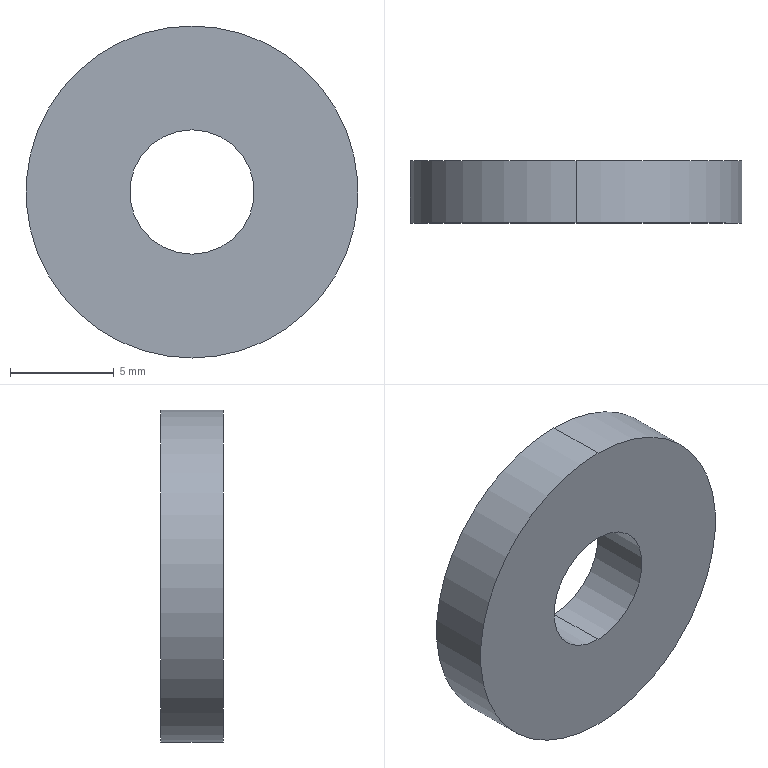Part | STEP file | PN_0004_default | 1 solid | 6 faces | box 16 x 3 x 16 mm | volume 518.363 mm3 | cylinder 4 | plane 2 | commonest cylinder face diameters 6 x2 16 x2
STEP:
#1=CARTESIAN_POINT('',(0.,0.,0.));
#2=DIRECTION('',(0.,0.,1.));
#3=DIRECTION('',(1.,0.,0.));
#4=AXIS2_PLACEMENT_3D('',#1,#2,#3);
#5=CARTESIAN_POINT('',(0.,3.,-3.));
#6=VERTEX_POINT('',#5);
#7=CARTESIAN_POINT('',(0.,0.,-3.));
#8=VERTEX_POINT('',#7);
#9=CARTESIAN_POINT('',(0.,3.,-3.));
#10=DIRECTION('',(0.,-1.,0.));
#11=VECTOR('',#10,1.);
#12=LINE('',#9,#11);
#13=CARTESIAN_POINT('',(0.,3.,0.));
#14=DIRECTION('',(0.,-1.,0.));
#15=DIRECTION('',(0.,0.,-1.));
#16=AXIS2_PLACEMENT_3D('',#13,#14,#15);
#17=CYLINDRICAL_SURFACE('',#16,3.);
#18=CARTESIAN_POINT('',(6.283,0.));
#19=DIRECTION('',(0.,1.));
#20=VECTOR('',#19,1.);
#21=LINE('',#18,#20);
#22=(GEOMETRIC_REPRESENTATION_CONTEXT(2)PARAMETRIC_REPRESENTATION_CONTEXT()REPRESENTATION_CONTEXT('',''));
#23=DEFINITIONAL_REPRESENTATION('',(#21),#22);
#24=PCURVE('',#17,#23);
#25=CARTESIAN_POINT('',(0.,3.,0.));
#26=DIRECTION('',(0.,-1.,0.));
#27=DIRECTION('',(0.,0.,-1.));
#28=AXIS2_PLACEMENT_3D('',#25,#26,#27);
#29=CYLINDRICAL_SURFACE('',#28,3.);
#30=CARTESIAN_POINT('',(0.,0.));
#31=DIRECTION('',(0.,1.));
#32=VECTOR('',#31,1.);
#33=LINE('',#30,#32);
#34=(GEOMETRIC_REPRESENTATION_CONTEXT(2)PARAMETRIC_REPRESENTATION_CONTEXT()REPRESENTATION_CONTEXT('',''));
#35=DEFINITIONAL_REPRESENTATION('',(#33),#34);
#36=PCURVE('',#29,#35);
#37=SURFACE_CURVE('',#12,(#24,#36),.PCURVE_S1.);
#38=EDGE_CURVE('',#6,#8,#37,.T.);
#39=ORIENTED_EDGE('',*,*,#38,.T.);
#40=CARTESIAN_POINT('',(0.,0.,3.));
#41=VERTEX_POINT('',#40);
#42=CARTESIAN_POINT('',(0.,0.,0.));
#43=DIRECTION('',(0.,1.,0.));
#44=DIRECTION('',(0.,0.,1.));
#45=AXIS2_PLACEMENT_3D('',#42,#43,#44);
#46=CIRCLE('',#45,3.);
#47=CARTESIAN_POINT('',(9.425,3.));
#48=DIRECTION('',(-1.,0.));
#49=VECTOR('',#48,1.);
#50=LINE('',#47,#49);
#51=(GEOMETRIC_REPRESENTATION_CONTEXT(2)PARAMETRIC_REPRESENTATION_CONTEXT()REPRESENTATION_CONTEXT('',''));
#52=DEFINITIONAL_REPRESENTATION('',(#50),#51);
#53=PCURVE('',#17,#52);
#54=CARTESIAN_POINT('',(0.,0.,0.));
#55=DIRECTION('',(0.,1.,0.));
#56=DIRECTION('',(0.,0.,1.));
#57=AXIS2_PLACEMENT_3D('',#54,#55,#56);
#58=PLANE('',#57);
#59=CARTESIAN_POINT('',(0.,0.));
#60=DIRECTION('',(1.,0.));
#61=AXIS2_PLACEMENT_2D('',#59,#60);
#62=CIRCLE('',#61,3.);
#63=(GEOMETRIC_REPRESENTATION_CONTEXT(2)PARAMETRIC_REPRESENTATION_CONTEXT()REPRESENTATION_CONTEXT('',''));
#64=DEFINITIONAL_REPRESENTATION('',(#62),#63);
#65=PCURVE('',#58,#64);
#66=SURFACE_CURVE('',#46,(#53,#65),.PCURVE_S1.);
#67=EDGE_CURVE('',#8,#41,#66,.T.);
#68=ORIENTED_EDGE('',*,*,#67,.T.);
#69=CARTESIAN_POINT('',(0.,3.,3.));
#70=VERTEX_POINT('',#69);
#71=CARTESIAN_POINT('',(0.,3.,3.));
#72=DIRECTION('',(0.,-1.,0.));
#73=VECTOR('',#72,1.);
#74=LINE('',#71,#73);
#75=CARTESIAN_POINT('',(3.142,0.));
#76=DIRECTION('',(0.,1.));
#77=VECTOR('',#76,1.);
#78=LINE('',#75,#77);
#79=(GEOMETRIC_REPRESENTATION_CONTEXT(2)PARAMETRIC_REPRESENTATION_CONTEXT()REPRESENTATION_CONTEXT('',''));
#80=DEFINITIONAL_REPRESENTATION('',(#78),#79);
#81=PCURVE('',#17,#80);
#82=CARTESIAN_POINT('',(3.142,0.));
#83=DIRECTION('',(0.,1.));
#84=VECTOR('',#83,1.);
#85=LINE('',#82,#84);
#86=(GEOMETRIC_REPRESENTATION_CONTEXT(2)PARAMETRIC_REPRESENTATION_CONTEXT()REPRESENTATION_CONTEXT('',''));
#87=DEFINITIONAL_REPRESENTATION('',(#85),#86);
#88=PCURVE('',#29,#87);
#89=SURFACE_CURVE('',#74,(#81,#88),.PCURVE_S1.);
#90=EDGE_CURVE('',#70,#41,#89,.T.);
#91=ORIENTED_EDGE('',*,*,#90,.F.);
#92=CARTESIAN_POINT('',(0.,3.,0.));
#93=DIRECTION('',(0.,1.,0.));
#94=DIRECTION('',(0.,0.,1.));
#95=AXIS2_PLACEMENT_3D('',#92,#93,#94);
#96=CIRCLE('',#95,3.);
#97=CARTESIAN_POINT('',(9.425,0.));
#98=DIRECTION('',(-1.,0.));
#99=VECTOR('',#98,1.);
#100=LINE('',#97,#99);
#101=(GEOMETRIC_REPRESENTATION_CONTEXT(2)PARAMETRIC_REPRESENTATION_CONTEXT()REPRESENTATION_CONTEXT('',''));
#102=DEFINITIONAL_REPRESENTATION('',(#100),#101);
#103=PCURVE('',#17,#102);
#104=CARTESIAN_POINT('',(0.,3.,0.));
#105=DIRECTION('',(0.,1.,0.));
#106=DIRECTION('',(0.,0.,1.));
#107=AXIS2_PLACEMENT_3D('',#104,#105,#106);
#108=PLANE('',#107);
#109=CARTESIAN_POINT('',(0.,0.));
#110=DIRECTION('',(1.,0.));
#111=AXIS2_PLACEMENT_2D('',#109,#110);
#112=CIRCLE('',#111,3.);
#113=(GEOMETRIC_REPRESENTATION_CONTEXT(2)PARAMETRIC_REPRESENTATION_CONTEXT()REPRESENTATION_CONTEXT('',''));
#114=DEFINITIONAL_REPRESENTATION('',(#112),#113);
#115=PCURVE('',#108,#114);
#116=SURFACE_CURVE('',#96,(#103,#115),.PCURVE_S1.);
#117=EDGE_CURVE('',#6,#70,#116,.T.);
#118=ORIENTED_EDGE('',*,*,#117,.F.);
#119=EDGE_LOOP('',(#39,#68,#91,#118));
#120=FACE_BOUND('',#119,.F.);
#121=ADVANCED_FACE('',(#120),#17,.F.);
#122=CARTESIAN_POINT('',(0.,3.,8.));
#123=VERTEX_POINT('',#122);
#124=CARTESIAN_POINT('',(0.,3.,-8.));
#125=VERTEX_POINT('',#124);
#126=CARTESIAN_POINT('',(0.,3.,0.));
#127=DIRECTION('',(0.,1.,0.));
#128=DIRECTION('',(0.,0.,1.));
#129=AXIS2_PLACEMENT_3D('',#126,#127,#128);
#130=CIRCLE('',#129,8.);
#131=CARTESIAN_POINT('',(0.,3.,0.));
#132=DIRECTION('',(0.,-1.,0.));
#133=DIRECTION('',(0.,0.,-1.));
#134=AXIS2_PLACEMENT_3D('',#131,#132,#133);
#135=CYLINDRICAL_SURFACE('',#134,8.);
#136=CARTESIAN_POINT('',(3.142,0.));
#137=DIRECTION('',(-1.,0.));
#138=VECTOR('',#137,1.);
#139=LINE('',#136,#138);
#140=(GEOMETRIC_REPRESENTATION_CONTEXT(2)PARAMETRIC_REPRESENTATION_CONTEXT()REPRESENTATION_CONTEXT('',''));
#141=DEFINITIONAL_REPRESENTATION('',(#139),#140);
#142=PCURVE('',#135,#141);
#143=CARTESIAN_POINT('',(0.,0.));
#144=DIRECTION('',(1.,0.));
#145=AXIS2_PLACEMENT_2D('',#143,#144);
#146=CIRCLE('',#145,8.);
#147=(GEOMETRIC_REPRESENTATION_CONTEXT(2)PARAMETRIC_REPRESENTATION_CONTEXT()REPRESENTATION_CONTEXT('',''));
#148=DEFINITIONAL_REPRESENTATION('',(#146),#147);
#149=PCURVE('',#108,#148);
#150=SURFACE_CURVE('',#130,(#142,#149),.PCURVE_S1.);
#151=EDGE_CURVE('',#123,#125,#150,.T.);
#152=ORIENTED_EDGE('',*,*,#151,.F.);
#153=CARTESIAN_POINT('',(0.,0.,8.));
#154=VERTEX_POINT('',#153);
#155=CARTESIAN_POINT('',(0.,3.,8.));
#156=DIRECTION('',(0.,-1.,0.));
#157=VECTOR('',#156,1.);
#158=LINE('',#155,#157);
#159=CARTESIAN_POINT('',(3.142,0.));
#160=DIRECTION('',(0.,1.));
#161=VECTOR('',#160,1.);
#162=LINE('',#159,#161);
#163=(GEOMETRIC_REPRESENTATION_CONTEXT(2)PARAMETRIC_REPRESENTATION_CONTEXT()REPRESENTATION_CONTEXT('',''));
#164=DEFINITIONAL_REPRESENTATION('',(#162),#163);
#165=PCURVE('',#135,#164);
#166=CARTESIAN_POINT('',(0.,3.,0.));
#167=DIRECTION('',(0.,-1.,0.));
#168=DIRECTION('',(0.,0.,-1.));
#169=AXIS2_PLACEMENT_3D('',#166,#167,#168);
#170=CYLINDRICAL_SURFACE('',#169,8.);
#171=CARTESIAN_POINT('',(3.142,0.));
#172=DIRECTION('',(0.,1.));
#173=VECTOR('',#172,1.);
#174=LINE('',#171,#173);
#175=(GEOMETRIC_REPRESENTATION_CONTEXT(2)PARAMETRIC_REPRESENTATION_CONTEXT()REPRESENTATION_CONTEXT('',''));
#176=DEFINITIONAL_REPRESENTATION('',(#174),#175);
#177=PCURVE('',#170,#176);
#178=SURFACE_CURVE('',#158,(#165,#177),.PCURVE_S1.);
#179=EDGE_CURVE('',#123,#154,#178,.T.);
#180=ORIENTED_EDGE('',*,*,#179,.T.);
#181=CARTESIAN_POINT('',(0.,0.,-8.));
#182=VERTEX_POINT('',#181);
#183=CARTESIAN_POINT('',(0.,0.,0.));
#184=DIRECTION('',(0.,1.,0.));
#185=DIRECTION('',(0.,0.,1.));
#186=AXIS2_PLACEMENT_3D('',#183,#184,#185);
#187=CIRCLE('',#186,8.);
#188=CARTESIAN_POINT('',(3.142,3.));
#189=DIRECTION('',(-1.,0.));
#190=VECTOR('',#189,1.);
#191=LINE('',#188,#190);
#192=(GEOMETRIC_REPRESENTATION_CONTEXT(2)PARAMETRIC_REPRESENTATION_CONTEXT()REPRESENTATION_CONTEXT('',''));
#193=DEFINITIONAL_REPRESENTATION('',(#191),#192);
#194=PCURVE('',#135,#193);
#195=CARTESIAN_POINT('',(0.,0.));
#196=DIRECTION('',(1.,0.));
#197=AXIS2_PLACEMENT_2D('',#195,#196);
#198=CIRCLE('',#197,8.);
#199=(GEOMETRIC_REPRESENTATION_CONTEXT(2)PARAMETRIC_REPRESENTATION_CONTEXT()REPRESENTATION_CONTEXT('',''));
#200=DEFINITIONAL_REPRESENTATION('',(#198),#199);
#201=PCURVE('',#58,#200);
#202=SURFACE_CURVE('',#187,(#194,#201),.PCURVE_S1.);
#203=EDGE_CURVE('',#154,#182,#202,.T.);
#204=ORIENTED_EDGE('',*,*,#203,.T.);
#205=CARTESIAN_POINT('',(0.,3.,-8.));
#206=DIRECTION('',(0.,-1.,0.));
#207=VECTOR('',#206,1.);
#208=LINE('',#205,#207);
#209=CARTESIAN_POINT('',(0.,0.));
#210=DIRECTION('',(0.,1.));
#211=VECTOR('',#210,1.);
#212=LINE('',#209,#211);
#213=(GEOMETRIC_REPRESENTATION_CONTEXT(2)PARAMETRIC_REPRESENTATION_CONTEXT()REPRESENTATION_CONTEXT('',''));
#214=DEFINITIONAL_REPRESENTATION('',(#212),#213);
#215=PCURVE('',#135,#214);
#216=CARTESIAN_POINT('',(6.283,0.));
#217=DIRECTION('',(0.,1.));
#218=VECTOR('',#217,1.);
#219=LINE('',#216,#218);
#220=(GEOMETRIC_REPRESENTATION_CONTEXT(2)PARAMETRIC_REPRESENTATION_CONTEXT()REPRESENTATION_CONTEXT('',''));
#221=DEFINITIONAL_REPRESENTATION('',(#219),#220);
#222=PCURVE('',#170,#221);
#223=SURFACE_CURVE('',#208,(#215,#222),.PCURVE_S1.);
#224=EDGE_CURVE('',#125,#182,#223,.T.);
#225=ORIENTED_EDGE('',*,*,#224,.F.);
#226=EDGE_LOOP('',(#152,#180,#204,#225));
#227=FACE_BOUND('',#226,.T.);
#228=ADVANCED_FACE('',(#227),#135,.T.);
#229=CARTESIAN_POINT('',(0.,3.,0.));
#230=DIRECTION('',(0.,1.,0.));
#231=DIRECTION('',(0.,0.,1.));
#232=AXIS2_PLACEMENT_3D('',#229,#230,#231);
#233=CIRCLE('',#232,8.);
#234=CARTESIAN_POINT('',(0.,0.));
#235=DIRECTION('',(1.,0.));
#236=AXIS2_PLACEMENT_2D('',#234,#235);
#237=CIRCLE('',#236,8.);
#238=(GEOMETRIC_REPRESENTATION_CONTEXT(2)PARAMETRIC_REPRESENTATION_CONTEXT()REPRESENTATION_CONTEXT('',''));
#239=DEFINITIONAL_REPRESENTATION('',(#237),#238);
#240=PCURVE('',#108,#239);
#241=CARTESIAN_POINT('',(9.425,0.));
#242=DIRECTION('',(-1.,0.));
#243=VECTOR('',#242,1.);
#244=LINE('',#241,#243);
#245=(GEOMETRIC_REPRESENTATION_CONTEXT(2)PARAMETRIC_REPRESENTATION_CONTEXT()REPRESENTATION_CONTEXT('',''));
#246=DEFINITIONAL_REPRESENTATION('',(#244),#245);
#247=PCURVE('',#170,#246);
#248=SURFACE_CURVE('',#233,(#240,#247),.PCURVE_S1.);
#249=EDGE_CURVE('',#125,#123,#248,.T.);
#250=ORIENTED_EDGE('',*,*,#249,.T.);
#251=ORIENTED_EDGE('',*,*,#151,.T.);
#252=EDGE_LOOP('',(#250,#251));
#253=FACE_BOUND('',#252,.T.);
#254=ORIENTED_EDGE('',*,*,#117,.F.);
#255=CARTESIAN_POINT('',(0.,3.,0.));
#256=DIRECTION('',(0.,1.,0.));
#257=DIRECTION('',(0.,0.,1.));
#258=AXIS2_PLACEMENT_3D('',#255,#256,#257);
#259=CIRCLE('',#258,3.);
#260=CARTESIAN_POINT('',(0.,0.));
#261=DIRECTION('',(1.,0.));
#262=AXIS2_PLACEMENT_2D('',#260,#261);
#263=CIRCLE('',#262,3.);
#264=(GEOMETRIC_REPRESENTATION_CONTEXT(2)PARAMETRIC_REPRESENTATION_CONTEXT()REPRESENTATION_CONTEXT('',''));
#265=DEFINITIONAL_REPRESENTATION('',(#263),#264);
#266=PCURVE('',#108,#265);
#267=CARTESIAN_POINT('',(3.142,0.));
#268=DIRECTION('',(-1.,0.));
#269=VECTOR('',#268,1.);
#270=LINE('',#267,#269);
#271=(GEOMETRIC_REPRESENTATION_CONTEXT(2)PARAMETRIC_REPRESENTATION_CONTEXT()REPRESENTATION_CONTEXT('',''));
#272=DEFINITIONAL_REPRESENTATION('',(#270),#271);
#273=PCURVE('',#29,#272);
#274=SURFACE_CURVE('',#259,(#266,#273),.PCURVE_S1.);
#275=EDGE_CURVE('',#70,#6,#274,.T.);
#276=ORIENTED_EDGE('',*,*,#275,.F.);
#277=EDGE_LOOP('',(#254,#276));
#278=FACE_BOUND('',#277,.T.);
#279=ADVANCED_FACE('',(#253,#278),#108,.T.);
#280=CARTESIAN_POINT('',(0.,0.,0.));
#281=DIRECTION('',(0.,1.,0.));
#282=DIRECTION('',(0.,0.,1.));
#283=AXIS2_PLACEMENT_3D('',#280,#281,#282);
#284=CIRCLE('',#283,8.);
#285=CARTESIAN_POINT('',(0.,0.));
#286=DIRECTION('',(1.,0.));
#287=AXIS2_PLACEMENT_2D('',#285,#286);
#288=CIRCLE('',#287,8.);
#289=(GEOMETRIC_REPRESENTATION_CONTEXT(2)PARAMETRIC_REPRESENTATION_CONTEXT()REPRESENTATION_CONTEXT('',''));
#290=DEFINITIONAL_REPRESENTATION('',(#288),#289);
#291=PCURVE('',#58,#290);
#292=CARTESIAN_POINT('',(9.425,3.));
#293=DIRECTION('',(-1.,0.));
#294=VECTOR('',#293,1.);
#295=LINE('',#292,#294);
#296=(GEOMETRIC_REPRESENTATION_CONTEXT(2)PARAMETRIC_REPRESENTATION_CONTEXT()REPRESENTATION_CONTEXT('',''));
#297=DEFINITIONAL_REPRESENTATION('',(#295),#296);
#298=PCURVE('',#170,#297);
#299=SURFACE_CURVE('',#284,(#291,#298),.PCURVE_S1.);
#300=EDGE_CURVE('',#182,#154,#299,.T.);
#301=ORIENTED_EDGE('',*,*,#300,.F.);
#302=ORIENTED_EDGE('',*,*,#203,.F.);
#303=EDGE_LOOP('',(#301,#302));
#304=FACE_BOUND('',#303,.T.);
#305=ORIENTED_EDGE('',*,*,#67,.T.);
#306=CARTESIAN_POINT('',(0.,0.,0.));
#307=DIRECTION('',(0.,1.,0.));
#308=DIRECTION('',(0.,0.,1.));
#309=AXIS2_PLACEMENT_3D('',#306,#307,#308);
#310=CIRCLE('',#309,3.);
#311=CARTESIAN_POINT('',(0.,0.));
#312=DIRECTION('',(1.,0.));
#313=AXIS2_PLACEMENT_2D('',#311,#312);
#314=CIRCLE('',#313,3.);
#315=(GEOMETRIC_REPRESENTATION_CONTEXT(2)PARAMETRIC_REPRESENTATION_CONTEXT()REPRESENTATION_CONTEXT('',''));
#316=DEFINITIONAL_REPRESENTATION('',(#314),#315);
#317=PCURVE('',#58,#316);
#318=CARTESIAN_POINT('',(3.142,3.));
#319=DIRECTION('',(-1.,0.));
#320=VECTOR('',#319,1.);
#321=LINE('',#318,#320);
#322=(GEOMETRIC_REPRESENTATION_CONTEXT(2)PARAMETRIC_REPRESENTATION_CONTEXT()REPRESENTATION_CONTEXT('',''));
#323=DEFINITIONAL_REPRESENTATION('',(#321),#322);
#324=PCURVE('',#29,#323);
#325=SURFACE_CURVE('',#310,(#317,#324),.PCURVE_S1.);
#326=EDGE_CURVE('',#41,#8,#325,.T.);
#327=ORIENTED_EDGE('',*,*,#326,.T.);
#328=EDGE_LOOP('',(#305,#327));
#329=FACE_BOUND('',#328,.T.);
#330=ADVANCED_FACE('',(#304,#329),#58,.F.);
#331=ORIENTED_EDGE('',*,*,#179,.F.);
#332=ORIENTED_EDGE('',*,*,#249,.F.);
#333=ORIENTED_EDGE('',*,*,#224,.T.);
#334=ORIENTED_EDGE('',*,*,#300,.T.);
#335=EDGE_LOOP('',(#331,#332,#333,#334));
#336=FACE_BOUND('',#335,.T.);
#337=ADVANCED_FACE('',(#336),#170,.T.);
#338=ORIENTED_EDGE('',*,*,#326,.T.);
#339=ORIENTED_EDGE('',*,*,#38,.F.);
#340=ORIENTED_EDGE('',*,*,#275,.F.);
#341=ORIENTED_EDGE('',*,*,#90,.T.);
#342=EDGE_LOOP('',(#338,#339,#340,#341));
#343=FACE_BOUND('',#342,.F.);
#344=ADVANCED_FACE('',(#343),#29,.F.);
#345=CLOSED_SHELL('',(#121,#228,#279,#330,#337,#344));
#346=MANIFOLD_SOLID_BREP('',#345);
#347=(LENGTH_UNIT()NAMED_UNIT(*)SI_UNIT(.MILLI.,.METRE.));
#348=UNCERTAINTY_MEASURE_WITH_UNIT(LENGTH_MEASURE(0.0000001),#347,'','');
#349=(NAMED_UNIT(*)PLANE_ANGLE_UNIT()SI_UNIT($,.RADIAN.));
#350=(NAMED_UNIT(*)SI_UNIT($,.STERADIAN.)SOLID_ANGLE_UNIT());
#351=(GEOMETRIC_REPRESENTATION_CONTEXT(3)GLOBAL_UNCERTAINTY_ASSIGNED_CONTEXT((#348))GLOBAL_UNIT_ASSIGNED_CONTEXT((#347,#349,#350))REPRESENTATION_CONTEXT('',''));
#352=ADVANCED_BREP_SHAPE_REPRESENTATION('',(#4,#346),#351);